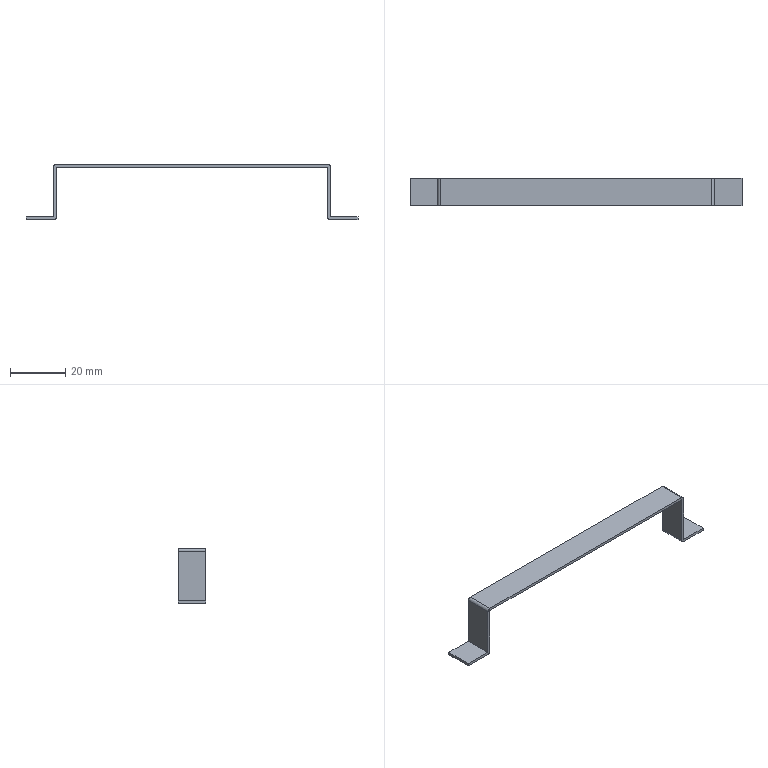Part | STEP file | RJWD-DY-0101_20001 | 1 solid | 18 faces | box 120 x 10 x 20 mm | volume 1571 mm3 | plane 14 | cylinder 4 | commonest cylinder face diameters 2.004 x3 2 x1
STEP:
#1=CARTESIAN_POINT('',(0.,0.,0.));
#2=DIRECTION('',(0.,0.,1.));
#3=DIRECTION('',(1.,0.,0.));
#4=AXIS2_PLACEMENT_3D('',#1,#2,#3);
#5=CARTESIAN_POINT('',(-930.573,5381.573,97.644));
#6=VERTEX_POINT('',#5);
#7=CARTESIAN_POINT('',(-931.573,5381.573,98.644));
#8=VERTEX_POINT('',#7);
#9=CARTESIAN_POINT('',(-931.573,5381.573,97.644));
#10=DIRECTION('',(0.,-1.,0.));
#11=DIRECTION('',(1.,0.,0.));
#12=AXIS2_PLACEMENT_3D('',#9,#10,#11);
#13=CIRCLE('',#12,1.);
#14=CARTESIAN_POINT('',(-1040.573,5381.573,97.644));
#15=DIRECTION('',(0.,-1.,0.));
#16=DIRECTION('',(0.,0.,-1.));
#17=AXIS2_PLACEMENT_3D('',#14,#15,#16);
#18=PLANE('',#17);
#19=CARTESIAN_POINT('',(0.,109.));
#20=DIRECTION('',(0.,1.));
#21=AXIS2_PLACEMENT_2D('',#19,#20);
#22=CIRCLE('',#21,1.);
#23=(GEOMETRIC_REPRESENTATION_CONTEXT(2)PARAMETRIC_REPRESENTATION_CONTEXT()REPRESENTATION_CONTEXT('',''));
#24=DEFINITIONAL_REPRESENTATION('',(#22),#23);
#25=PCURVE('',#18,#24);
#26=CARTESIAN_POINT('',(-931.573,5345.501,97.644));
#27=DIRECTION('',(0.,1.,0.));
#28=DIRECTION('',(0.,0.,1.));
#29=AXIS2_PLACEMENT_3D('',#26,#27,#28);
#30=CYLINDRICAL_SURFACE('',#29,1.);
#31=CARTESIAN_POINT('',(1.571,36.072));
#32=DIRECTION('',(-1.,0.));
#33=VECTOR('',#32,1.);
#34=LINE('',#31,#33);
#35=(GEOMETRIC_REPRESENTATION_CONTEXT(2)PARAMETRIC_REPRESENTATION_CONTEXT()REPRESENTATION_CONTEXT('',''));
#36=DEFINITIONAL_REPRESENTATION('',(#34),#35);
#37=PCURVE('',#30,#36);
#38=SURFACE_CURVE('',#13,(#25,#37),.PCURVE_S1.);
#39=EDGE_CURVE('',#6,#8,#38,.T.);
#40=ORIENTED_EDGE('',*,*,#39,.F.);
#41=CARTESIAN_POINT('',(-930.573,5381.573,79.644));
#42=VERTEX_POINT('',#41);
#43=CARTESIAN_POINT('',(-930.573,5381.573,97.644));
#44=DIRECTION('',(0.,0.,-1.));
#45=VECTOR('',#44,1.);
#46=LINE('',#43,#45);
#47=CARTESIAN_POINT('',(0.,110.));
#48=DIRECTION('',(1.,0.));
#49=VECTOR('',#48,1.);
#50=LINE('',#47,#49);
#51=(GEOMETRIC_REPRESENTATION_CONTEXT(2)PARAMETRIC_REPRESENTATION_CONTEXT()REPRESENTATION_CONTEXT('',''));
#52=DEFINITIONAL_REPRESENTATION('',(#50),#51);
#53=PCURVE('',#18,#52);
#54=CARTESIAN_POINT('',(-930.573,-10.,0.));
#55=DIRECTION('',(1.,0.,0.));
#56=DIRECTION('',(0.,0.,-1.));
#57=AXIS2_PLACEMENT_3D('',#54,#55,#56);
#58=PLANE('',#57);
#59=CARTESIAN_POINT('',(-97.644,5391.573));
#60=DIRECTION('',(1.,0.));
#61=VECTOR('',#60,1.);
#62=LINE('',#59,#61);
#63=(GEOMETRIC_REPRESENTATION_CONTEXT(2)PARAMETRIC_REPRESENTATION_CONTEXT()REPRESENTATION_CONTEXT('',''));
#64=DEFINITIONAL_REPRESENTATION('',(#62),#63);
#65=PCURVE('',#58,#64);
#66=SURFACE_CURVE('',#46,(#53,#65),.PCURVE_S1.);
#67=EDGE_CURVE('',#6,#42,#66,.T.);
#68=ORIENTED_EDGE('',*,*,#67,.T.);
#69=CARTESIAN_POINT('',(-920.573,5381.573,79.644));
#70=VERTEX_POINT('',#69);
#71=CARTESIAN_POINT('',(-920.573,5381.573,79.644));
#72=DIRECTION('',(-1.,0.,0.));
#73=VECTOR('',#72,1.);
#74=LINE('',#71,#73);
#75=CARTESIAN_POINT('',(18.,120.));
#76=DIRECTION('',(0.,-1.));
#77=VECTOR('',#76,1.);
#78=LINE('',#75,#77);
#79=(GEOMETRIC_REPRESENTATION_CONTEXT(2)PARAMETRIC_REPRESENTATION_CONTEXT()REPRESENTATION_CONTEXT('',''));
#80=DEFINITIONAL_REPRESENTATION('',(#78),#79);
#81=PCURVE('',#18,#80);
#82=CARTESIAN_POINT('',(-110.,-10.,79.644));
#83=DIRECTION('',(0.,0.,1.));
#84=DIRECTION('',(1.,0.,0.));
#85=AXIS2_PLACEMENT_3D('',#82,#83,#84);
#86=PLANE('',#85);
#87=CARTESIAN_POINT('',(-810.573,5391.573));
#88=DIRECTION('',(-1.,0.));
#89=VECTOR('',#88,1.);
#90=LINE('',#87,#89);
#91=(GEOMETRIC_REPRESENTATION_CONTEXT(2)PARAMETRIC_REPRESENTATION_CONTEXT()REPRESENTATION_CONTEXT('',''));
#92=DEFINITIONAL_REPRESENTATION('',(#90),#91);
#93=PCURVE('',#86,#92);
#94=SURFACE_CURVE('',#74,(#81,#93),.PCURVE_S1.);
#95=EDGE_CURVE('',#70,#42,#94,.T.);
#96=ORIENTED_EDGE('',*,*,#95,.F.);
#97=CARTESIAN_POINT('',(-920.573,5381.573,78.644));
#98=VERTEX_POINT('',#97);
#99=CARTESIAN_POINT('',(-920.573,5381.573,79.644));
#100=DIRECTION('',(0.,0.,-1.));
#101=VECTOR('',#100,1.);
#102=LINE('',#99,#101);
#103=CARTESIAN_POINT('',(18.,120.));
#104=DIRECTION('',(1.,0.));
#105=VECTOR('',#104,1.);
#106=LINE('',#103,#105);
#107=(GEOMETRIC_REPRESENTATION_CONTEXT(2)PARAMETRIC_REPRESENTATION_CONTEXT()REPRESENTATION_CONTEXT('',''));
#108=DEFINITIONAL_REPRESENTATION('',(#106),#107);
#109=PCURVE('',#18,#108);
#110=CARTESIAN_POINT('',(-920.573,5371.573,78.644));
#111=DIRECTION('',(1.,0.,0.));
#112=DIRECTION('',(0.,0.,-1.));
#113=AXIS2_PLACEMENT_3D('',#110,#111,#112);
#114=PLANE('',#113);
#115=CARTESIAN_POINT('',(-1.,10.));
#116=DIRECTION('',(1.,0.));
#117=VECTOR('',#116,1.);
#118=LINE('',#115,#117);
#119=(GEOMETRIC_REPRESENTATION_CONTEXT(2)PARAMETRIC_REPRESENTATION_CONTEXT()REPRESENTATION_CONTEXT('',''));
#120=DEFINITIONAL_REPRESENTATION('',(#118),#119);
#121=PCURVE('',#114,#120);
#122=SURFACE_CURVE('',#102,(#109,#121),.PCURVE_S1.);
#123=EDGE_CURVE('',#70,#98,#122,.T.);
#124=ORIENTED_EDGE('',*,*,#123,.T.);
#125=CARTESIAN_POINT('',(-930.571,5381.573,78.644));
#126=VERTEX_POINT('',#125);
#127=CARTESIAN_POINT('',(-920.573,5381.573,78.644));
#128=DIRECTION('',(-1.,0.,0.));
#129=VECTOR('',#128,1.);
#130=LINE('',#127,#129);
#131=CARTESIAN_POINT('',(19.,120.));
#132=DIRECTION('',(0.,-1.));
#133=VECTOR('',#132,1.);
#134=LINE('',#131,#133);
#135=(GEOMETRIC_REPRESENTATION_CONTEXT(2)PARAMETRIC_REPRESENTATION_CONTEXT()REPRESENTATION_CONTEXT('',''));
#136=DEFINITIONAL_REPRESENTATION('',(#134),#135);
#137=PCURVE('',#18,#136);
#138=CARTESIAN_POINT('',(-110.,-10.,78.644));
#139=DIRECTION('',(0.,0.,1.));
#140=DIRECTION('',(1.,0.,0.));
#141=AXIS2_PLACEMENT_3D('',#138,#139,#140);
#142=PLANE('',#141);
#143=CARTESIAN_POINT('',(-810.573,5391.573));
#144=DIRECTION('',(-1.,0.));
#145=VECTOR('',#144,1.);
#146=LINE('',#143,#145);
#147=(GEOMETRIC_REPRESENTATION_CONTEXT(2)PARAMETRIC_REPRESENTATION_CONTEXT()REPRESENTATION_CONTEXT('',''));
#148=DEFINITIONAL_REPRESENTATION('',(#146),#147);
#149=PCURVE('',#142,#148);
#150=SURFACE_CURVE('',#130,(#137,#149),.PCURVE_S1.);
#151=EDGE_CURVE('',#98,#126,#150,.T.);
#152=ORIENTED_EDGE('',*,*,#151,.T.);
#153=CARTESIAN_POINT('',(-931.573,5381.573,79.646));
#154=VERTEX_POINT('',#153);
#155=CARTESIAN_POINT('',(-930.571,5381.573,79.646));
#156=DIRECTION('',(0.,-1.,0.));
#157=DIRECTION('',(-1.,0.,0.));
#158=AXIS2_PLACEMENT_3D('',#155,#156,#157);
#159=CIRCLE('',#158,1.002);
#160=CARTESIAN_POINT('',(17.998,110.002));
#161=DIRECTION('',(0.,-1.));
#162=AXIS2_PLACEMENT_2D('',#160,#161);
#163=CIRCLE('',#162,1.002);
#164=(GEOMETRIC_REPRESENTATION_CONTEXT(2)PARAMETRIC_REPRESENTATION_CONTEXT()REPRESENTATION_CONTEXT('',''));
#165=DEFINITIONAL_REPRESENTATION('',(#163),#164);
#166=PCURVE('',#18,#165);
#167=CARTESIAN_POINT('',(-930.571,5411.573,79.646));
#168=DIRECTION('',(0.,-1.,0.));
#169=DIRECTION('',(1.,0.,0.));
#170=AXIS2_PLACEMENT_3D('',#167,#168,#169);
#171=CYLINDRICAL_SURFACE('',#170,1.002);
#172=CARTESIAN_POINT('',(3.142,30.));
#173=DIRECTION('',(1.,0.));
#174=VECTOR('',#173,1.);
#175=LINE('',#172,#174);
#176=(GEOMETRIC_REPRESENTATION_CONTEXT(2)PARAMETRIC_REPRESENTATION_CONTEXT()REPRESENTATION_CONTEXT('',''));
#177=DEFINITIONAL_REPRESENTATION('',(#175),#176);
#178=PCURVE('',#171,#177);
#179=SURFACE_CURVE('',#159,(#166,#178),.PCURVE_S1.);
#180=EDGE_CURVE('',#154,#126,#179,.T.);
#181=ORIENTED_EDGE('',*,*,#180,.F.);
#182=CARTESIAN_POINT('',(-931.573,5381.573,97.644));
#183=VERTEX_POINT('',#182);
#184=CARTESIAN_POINT('',(-931.573,5381.573,79.646));
#185=DIRECTION('',(0.,0.,1.));
#186=VECTOR('',#185,1.);
#187=LINE('',#184,#186);
#188=CARTESIAN_POINT('',(17.998,109.));
#189=DIRECTION('',(-1.,0.));
#190=VECTOR('',#189,1.);
#191=LINE('',#188,#190);
#192=(GEOMETRIC_REPRESENTATION_CONTEXT(2)PARAMETRIC_REPRESENTATION_CONTEXT()REPRESENTATION_CONTEXT('',''));
#193=DEFINITIONAL_REPRESENTATION('',(#191),#192);
#194=PCURVE('',#18,#193);
#195=CARTESIAN_POINT('',(-931.573,-10.,0.));
#196=DIRECTION('',(1.,0.,0.));
#197=DIRECTION('',(0.,0.,-1.));
#198=AXIS2_PLACEMENT_3D('',#195,#196,#197);
#199=PLANE('',#198);
#200=CARTESIAN_POINT('',(-79.646,5391.573));
#201=DIRECTION('',(-1.,0.));
#202=VECTOR('',#201,1.);
#203=LINE('',#200,#202);
#204=(GEOMETRIC_REPRESENTATION_CONTEXT(2)PARAMETRIC_REPRESENTATION_CONTEXT()REPRESENTATION_CONTEXT('',''));
#205=DEFINITIONAL_REPRESENTATION('',(#203),#204);
#206=PCURVE('',#199,#205);
#207=SURFACE_CURVE('',#187,(#194,#206),.PCURVE_S1.);
#208=EDGE_CURVE('',#154,#183,#207,.T.);
#209=ORIENTED_EDGE('',*,*,#208,.T.);
#210=CARTESIAN_POINT('',(-1029.573,5381.573,97.644));
#211=VERTEX_POINT('',#210);
#212=CARTESIAN_POINT('',(-931.573,5381.573,97.644));
#213=DIRECTION('',(-1.,0.,0.));
#214=VECTOR('',#213,1.);
#215=LINE('',#212,#214);
#216=CARTESIAN_POINT('',(0.,109.));
#217=DIRECTION('',(0.,-1.));
#218=VECTOR('',#217,1.);
#219=LINE('',#216,#218);
#220=(GEOMETRIC_REPRESENTATION_CONTEXT(2)PARAMETRIC_REPRESENTATION_CONTEXT()REPRESENTATION_CONTEXT('',''));
#221=DEFINITIONAL_REPRESENTATION('',(#219),#220);
#222=PCURVE('',#18,#221);
#223=CARTESIAN_POINT('',(0.,-10.,97.644));
#224=DIRECTION('',(0.,0.,1.));
#225=DIRECTION('',(1.,0.,0.));
#226=AXIS2_PLACEMENT_3D('',#223,#224,#225);
#227=PLANE('',#226);
#228=CARTESIAN_POINT('',(-931.573,5391.573));
#229=DIRECTION('',(-1.,0.));
#230=VECTOR('',#229,1.);
#231=LINE('',#228,#230);
#232=(GEOMETRIC_REPRESENTATION_CONTEXT(2)PARAMETRIC_REPRESENTATION_CONTEXT()REPRESENTATION_CONTEXT('',''));
#233=DEFINITIONAL_REPRESENTATION('',(#231),#232);
#234=PCURVE('',#227,#233);
#235=SURFACE_CURVE('',#215,(#222,#234),.PCURVE_S1.);
#236=EDGE_CURVE('',#183,#211,#235,.T.);
#237=ORIENTED_EDGE('',*,*,#236,.T.);
#238=CARTESIAN_POINT('',(-1029.573,5381.573,79.646));
#239=VERTEX_POINT('',#238);
#240=CARTESIAN_POINT('',(-1029.573,5381.573,79.646));
#241=DIRECTION('',(0.,0.,1.));
#242=VECTOR('',#241,1.);
#243=LINE('',#240,#242);
#244=CARTESIAN_POINT('',(17.998,11.));
#245=DIRECTION('',(-1.,0.));
#246=VECTOR('',#245,1.);
#247=LINE('',#244,#246);
#248=(GEOMETRIC_REPRESENTATION_CONTEXT(2)PARAMETRIC_REPRESENTATION_CONTEXT()REPRESENTATION_CONTEXT('',''));
#249=DEFINITIONAL_REPRESENTATION('',(#247),#248);
#250=PCURVE('',#18,#249);
#251=CARTESIAN_POINT('',(-1029.573,-10.,0.));
#252=DIRECTION('',(1.,0.,0.));
#253=DIRECTION('',(0.,0.,-1.));
#254=AXIS2_PLACEMENT_3D('',#251,#252,#253);
#255=PLANE('',#254);
#256=CARTESIAN_POINT('',(-79.646,5391.573));
#257=DIRECTION('',(-1.,0.));
#258=VECTOR('',#257,1.);
#259=LINE('',#256,#258);
#260=(GEOMETRIC_REPRESENTATION_CONTEXT(2)PARAMETRIC_REPRESENTATION_CONTEXT()REPRESENTATION_CONTEXT('',''));
#261=DEFINITIONAL_REPRESENTATION('',(#259),#260);
#262=PCURVE('',#255,#261);
#263=SURFACE_CURVE('',#243,(#250,#262),.PCURVE_S1.);
#264=EDGE_CURVE('',#239,#211,#263,.T.);
#265=ORIENTED_EDGE('',*,*,#264,.F.);
#266=CARTESIAN_POINT('',(-1030.575,5381.573,78.644));
#267=VERTEX_POINT('',#266);
#268=CARTESIAN_POINT('',(-1030.575,5381.573,79.646));
#269=DIRECTION('',(0.,-1.,0.));
#270=DIRECTION('',(0.,0.,-1.));
#271=AXIS2_PLACEMENT_3D('',#268,#269,#270);
#272=CIRCLE('',#271,1.002);
#273=CARTESIAN_POINT('',(17.998,9.998));
#274=DIRECTION('',(1.,0.));
#275=AXIS2_PLACEMENT_2D('',#273,#274);
#276=CIRCLE('',#275,1.002);
#277=(GEOMETRIC_REPRESENTATION_CONTEXT(2)PARAMETRIC_REPRESENTATION_CONTEXT()REPRESENTATION_CONTEXT('',''));
#278=DEFINITIONAL_REPRESENTATION('',(#276),#277);
#279=PCURVE('',#18,#278);
#280=CARTESIAN_POINT('',(-1030.575,5371.573,79.646));
#281=DIRECTION('',(0.,1.,0.));
#282=DIRECTION('',(-1.,0.,0.));
#283=AXIS2_PLACEMENT_3D('',#280,#281,#282);
#284=CYLINDRICAL_SURFACE('',#283,1.002);
#285=CARTESIAN_POINT('',(4.712,10.));
#286=DIRECTION('',(-1.,0.));
#287=VECTOR('',#286,1.);
#288=LINE('',#285,#287);
#289=(GEOMETRIC_REPRESENTATION_CONTEXT(2)PARAMETRIC_REPRESENTATION_CONTEXT()REPRESENTATION_CONTEXT('',''));
#290=DEFINITIONAL_REPRESENTATION('',(#288),#289);
#291=PCURVE('',#284,#290);
#292=SURFACE_CURVE('',#272,(#279,#291),.PCURVE_S1.);
#293=EDGE_CURVE('',#267,#239,#292,.T.);
#294=ORIENTED_EDGE('',*,*,#293,.F.);
#295=CARTESIAN_POINT('',(-1040.573,5381.573,78.644));
#296=VERTEX_POINT('',#295);
#297=CARTESIAN_POINT('',(-1040.573,5381.573,78.644));
#298=DIRECTION('',(1.,0.,0.));
#299=VECTOR('',#298,1.);
#300=LINE('',#297,#299);
#301=CARTESIAN_POINT('',(19.,0.));
#302=DIRECTION('',(0.,1.));
#303=VECTOR('',#302,1.);
#304=LINE('',#301,#303);
#305=(GEOMETRIC_REPRESENTATION_CONTEXT(2)PARAMETRIC_REPRESENTATION_CONTEXT()REPRESENTATION_CONTEXT('',''));
#306=DEFINITIONAL_REPRESENTATION('',(#304),#305);
#307=PCURVE('',#18,#306);
#308=CARTESIAN_POINT('',(10.,-10.,78.644));
#309=DIRECTION('',(0.,0.,-1.));
#310=DIRECTION('',(-1.,0.,0.));
#311=AXIS2_PLACEMENT_3D('',#308,#309,#310);
#312=PLANE('',#311);
#313=CARTESIAN_POINT('',(1050.573,5391.573));
#314=DIRECTION('',(-1.,0.));
#315=VECTOR('',#314,1.);
#316=LINE('',#313,#315);
#317=(GEOMETRIC_REPRESENTATION_CONTEXT(2)PARAMETRIC_REPRESENTATION_CONTEXT()REPRESENTATION_CONTEXT('',''));
#318=DEFINITIONAL_REPRESENTATION('',(#316),#317);
#319=PCURVE('',#312,#318);
#320=SURFACE_CURVE('',#300,(#307,#319),.PCURVE_S1.);
#321=EDGE_CURVE('',#296,#267,#320,.T.);
#322=ORIENTED_EDGE('',*,*,#321,.F.);
#323=CARTESIAN_POINT('',(-1040.573,5381.573,79.644));
#324=VERTEX_POINT('',#323);
#325=CARTESIAN_POINT('',(-1040.573,5381.573,79.644));
#326=DIRECTION('',(0.,0.,-1.));
#327=VECTOR('',#326,1.);
#328=LINE('',#325,#327);
#329=CARTESIAN_POINT('',(18.,0.));
#330=DIRECTION('',(1.,0.));
#331=VECTOR('',#330,1.);
#332=LINE('',#329,#331);
#333=(GEOMETRIC_REPRESENTATION_CONTEXT(2)PARAMETRIC_REPRESENTATION_CONTEXT()REPRESENTATION_CONTEXT('',''));
#334=DEFINITIONAL_REPRESENTATION('',(#332),#333);
#335=PCURVE('',#18,#334);
#336=CARTESIAN_POINT('',(-1040.573,5371.573,78.644));
#337=DIRECTION('',(1.,0.,0.));
#338=DIRECTION('',(0.,0.,-1.));
#339=AXIS2_PLACEMENT_3D('',#336,#337,#338);
#340=PLANE('',#339);
#341=CARTESIAN_POINT('',(-1.,10.));
#342=DIRECTION('',(1.,0.));
#343=VECTOR('',#342,1.);
#344=LINE('',#341,#343);
#345=(GEOMETRIC_REPRESENTATION_CONTEXT(2)PARAMETRIC_REPRESENTATION_CONTEXT()REPRESENTATION_CONTEXT('',''));
#346=DEFINITIONAL_REPRESENTATION('',(#344),#345);
#347=PCURVE('',#340,#346);
#348=SURFACE_CURVE('',#328,(#335,#347),.PCURVE_S1.);
#349=EDGE_CURVE('',#324,#296,#348,.T.);
#350=ORIENTED_EDGE('',*,*,#349,.F.);
#351=CARTESIAN_POINT('',(-1030.573,5381.573,79.644));
#352=VERTEX_POINT('',#351);
#353=CARTESIAN_POINT('',(-1040.573,5381.573,79.644));
#354=DIRECTION('',(1.,0.,0.));
#355=VECTOR('',#354,1.);
#356=LINE('',#353,#355);
#357=CARTESIAN_POINT('',(18.,0.));
#358=DIRECTION('',(0.,1.));
#359=VECTOR('',#358,1.);
#360=LINE('',#357,#359);
#361=(GEOMETRIC_REPRESENTATION_CONTEXT(2)PARAMETRIC_REPRESENTATION_CONTEXT()REPRESENTATION_CONTEXT('',''));
#362=DEFINITIONAL_REPRESENTATION('',(#360),#361);
#363=PCURVE('',#18,#362);
#364=CARTESIAN_POINT('',(10.,-10.,79.644));
#365=DIRECTION('',(0.,0.,-1.));
#366=DIRECTION('',(-1.,0.,0.));
#367=AXIS2_PLACEMENT_3D('',#364,#365,#366);
#368=PLANE('',#367);
#369=CARTESIAN_POINT('',(1050.573,5391.573));
#370=DIRECTION('',(-1.,0.));
#371=VECTOR('',#370,1.);
#372=LINE('',#369,#371);
#373=(GEOMETRIC_REPRESENTATION_CONTEXT(2)PARAMETRIC_REPRESENTATION_CONTEXT()REPRESENTATION_CONTEXT('',''));
#374=DEFINITIONAL_REPRESENTATION('',(#372),#373);
#375=PCURVE('',#368,#374);
#376=SURFACE_CURVE('',#356,(#363,#375),.PCURVE_S1.);
#377=EDGE_CURVE('',#324,#352,#376,.T.);
#378=ORIENTED_EDGE('',*,*,#377,.T.);
#379=CARTESIAN_POINT('',(-1030.573,5381.573,97.642));
#380=VERTEX_POINT('',#379);
#381=CARTESIAN_POINT('',(-1030.573,5381.573,79.644));
#382=DIRECTION('',(0.,0.,1.));
#383=VECTOR('',#382,1.);
#384=LINE('',#381,#383);
#385=CARTESIAN_POINT('',(18.,10.));
#386=DIRECTION('',(-1.,0.));
#387=VECTOR('',#386,1.);
#388=LINE('',#385,#387);
#389=(GEOMETRIC_REPRESENTATION_CONTEXT(2)PARAMETRIC_REPRESENTATION_CONTEXT()REPRESENTATION_CONTEXT('',''));
#390=DEFINITIONAL_REPRESENTATION('',(#388),#389);
#391=PCURVE('',#18,#390);
#392=CARTESIAN_POINT('',(-1030.573,-10.,0.));
#393=DIRECTION('',(1.,0.,0.));
#394=DIRECTION('',(0.,0.,-1.));
#395=AXIS2_PLACEMENT_3D('',#392,#393,#394);
#396=PLANE('',#395);
#397=CARTESIAN_POINT('',(-79.644,5391.573));
#398=DIRECTION('',(-1.,0.));
#399=VECTOR('',#398,1.);
#400=LINE('',#397,#399);
#401=(GEOMETRIC_REPRESENTATION_CONTEXT(2)PARAMETRIC_REPRESENTATION_CONTEXT()REPRESENTATION_CONTEXT('',''));
#402=DEFINITIONAL_REPRESENTATION('',(#400),#401);
#403=PCURVE('',#396,#402);
#404=SURFACE_CURVE('',#384,(#391,#403),.PCURVE_S1.);
#405=EDGE_CURVE('',#352,#380,#404,.T.);
#406=ORIENTED_EDGE('',*,*,#405,.T.);
#407=CARTESIAN_POINT('',(-1029.571,5381.573,98.644));
#408=VERTEX_POINT('',#407);
#409=CARTESIAN_POINT('',(-1029.571,5381.573,97.642));
#410=DIRECTION('',(0.,-1.,0.));
#411=DIRECTION('',(0.,0.,1.));
#412=AXIS2_PLACEMENT_3D('',#409,#410,#411);
#413=CIRCLE('',#412,1.002);
#414=CARTESIAN_POINT('',(0.002,11.002));
#415=DIRECTION('',(-1.,0.));
#416=AXIS2_PLACEMENT_2D('',#414,#415);
#417=CIRCLE('',#416,1.002);
#418=(GEOMETRIC_REPRESENTATION_CONTEXT(2)PARAMETRIC_REPRESENTATION_CONTEXT()REPRESENTATION_CONTEXT('',''));
#419=DEFINITIONAL_REPRESENTATION('',(#417),#418);
#420=PCURVE('',#18,#419);
#421=CARTESIAN_POINT('',(-1029.571,5411.573,97.642));
#422=DIRECTION('',(0.,-1.,0.));
#423=DIRECTION('',(0.,0.,-1.));
#424=AXIS2_PLACEMENT_3D('',#421,#422,#423);
#425=CYLINDRICAL_SURFACE('',#424,1.002);
#426=CARTESIAN_POINT('',(3.142,30.));
#427=DIRECTION('',(1.,0.));
#428=VECTOR('',#427,1.);
#429=LINE('',#426,#428);
#430=(GEOMETRIC_REPRESENTATION_CONTEXT(2)PARAMETRIC_REPRESENTATION_CONTEXT()REPRESENTATION_CONTEXT('',''));
#431=DEFINITIONAL_REPRESENTATION('',(#429),#430);
#432=PCURVE('',#425,#431);
#433=SURFACE_CURVE('',#413,(#420,#432),.PCURVE_S1.);
#434=EDGE_CURVE('',#408,#380,#433,.T.);
#435=ORIENTED_EDGE('',*,*,#434,.F.);
#436=CARTESIAN_POINT('',(-1029.571,5381.573,98.644));
#437=DIRECTION('',(1.,0.,0.));
#438=VECTOR('',#437,1.);
#439=LINE('',#436,#438);
#440=CARTESIAN_POINT('',(-1.,11.002));
#441=DIRECTION('',(0.,1.));
#442=VECTOR('',#441,1.);
#443=LINE('',#440,#442);
#444=(GEOMETRIC_REPRESENTATION_CONTEXT(2)PARAMETRIC_REPRESENTATION_CONTEXT()REPRESENTATION_CONTEXT('',''));
#445=DEFINITIONAL_REPRESENTATION('',(#443),#444);
#446=PCURVE('',#18,#445);
#447=CARTESIAN_POINT('',(0.,-10.,98.644));
#448=DIRECTION('',(0.,0.,1.));
#449=DIRECTION('',(1.,0.,0.));
#450=AXIS2_PLACEMENT_3D('',#447,#448,#449);
#451=PLANE('',#450);
#452=CARTESIAN_POINT('',(-1029.571,5391.573));
#453=DIRECTION('',(1.,0.));
#454=VECTOR('',#453,1.);
#455=LINE('',#452,#454);
#456=(GEOMETRIC_REPRESENTATION_CONTEXT(2)PARAMETRIC_REPRESENTATION_CONTEXT()REPRESENTATION_CONTEXT('',''));
#457=DEFINITIONAL_REPRESENTATION('',(#455),#456);
#458=PCURVE('',#451,#457);
#459=SURFACE_CURVE('',#439,(#446,#458),.PCURVE_S1.);
#460=EDGE_CURVE('',#408,#8,#459,.T.);
#461=ORIENTED_EDGE('',*,*,#460,.T.);
#462=EDGE_LOOP('',(#40,#68,#96,#124,#152,#181,#209,#237,#265,#294,#322,#350,#378,#406,#435,#461));
#463=FACE_BOUND('',#462,.F.);
#464=ADVANCED_FACE('',(#463),#18,.T.);
#465=CARTESIAN_POINT('',(-931.573,5391.573,98.644));
#466=VERTEX_POINT('',#465);
#467=CARTESIAN_POINT('',(-931.573,5381.573,98.644));
#468=DIRECTION('',(0.,1.,0.));
#469=VECTOR('',#468,1.);
#470=LINE('',#467,#469);
#471=CARTESIAN_POINT('',(0.,36.072));
#472=DIRECTION('',(0.,1.));
#473=VECTOR('',#472,1.);
#474=LINE('',#471,#473);
#475=(GEOMETRIC_REPRESENTATION_CONTEXT(2)PARAMETRIC_REPRESENTATION_CONTEXT()REPRESENTATION_CONTEXT('',''));
#476=DEFINITIONAL_REPRESENTATION('',(#474),#475);
#477=PCURVE('',#30,#476);
#478=CARTESIAN_POINT('',(-931.573,5391.573));
#479=DIRECTION('',(0.,1.));
#480=VECTOR('',#479,1.);
#481=LINE('',#478,#480);
#482=(GEOMETRIC_REPRESENTATION_CONTEXT(2)PARAMETRIC_REPRESENTATION_CONTEXT()REPRESENTATION_CONTEXT('',''));
#483=DEFINITIONAL_REPRESENTATION('',(#481),#482);
#484=PCURVE('',#451,#483);
#485=SURFACE_CURVE('',#470,(#477,#484),.PCURVE_S1.);
#486=EDGE_CURVE('',#8,#466,#485,.T.);
#487=ORIENTED_EDGE('',*,*,#486,.F.);
#488=ORIENTED_EDGE('',*,*,#39,.F.);
#489=CARTESIAN_POINT('',(-930.573,5391.573,97.644));
#490=VERTEX_POINT('',#489);
#491=CARTESIAN_POINT('',(-930.573,5381.573,97.644));
#492=DIRECTION('',(0.,1.,0.));
#493=VECTOR('',#492,1.);
#494=LINE('',#491,#493);
#495=CARTESIAN_POINT('',(1.571,36.072));
#496=DIRECTION('',(0.,1.));
#497=VECTOR('',#496,1.);
#498=LINE('',#495,#497);
#499=(GEOMETRIC_REPRESENTATION_CONTEXT(2)PARAMETRIC_REPRESENTATION_CONTEXT()REPRESENTATION_CONTEXT('',''));
#500=DEFINITIONAL_REPRESENTATION('',(#498),#499);
#501=PCURVE('',#30,#500);
#502=CARTESIAN_POINT('',(-97.644,5391.573));
#503=DIRECTION('',(0.,1.));
#504=VECTOR('',#503,1.);
#505=LINE('',#502,#504);
#506=(GEOMETRIC_REPRESENTATION_CONTEXT(2)PARAMETRIC_REPRESENTATION_CONTEXT()REPRESENTATION_CONTEXT('',''));
#507=DEFINITIONAL_REPRESENTATION('',(#505),#506);
#508=PCURVE('',#58,#507);
#509=SURFACE_CURVE('',#494,(#501,#508),.PCURVE_S1.);
#510=EDGE_CURVE('',#6,#490,#509,.T.);
#511=ORIENTED_EDGE('',*,*,#510,.T.);
#512=CARTESIAN_POINT('',(-931.573,5391.573,97.644));
#513=DIRECTION('',(0.,1.,0.));
#514=DIRECTION('',(0.,0.,1.));
#515=AXIS2_PLACEMENT_3D('',#512,#513,#514);
#516=CIRCLE('',#515,1.);
#517=CARTESIAN_POINT('',(0.,46.072));
#518=DIRECTION('',(1.,0.));
#519=VECTOR('',#518,1.);
#520=LINE('',#517,#519);
#521=(GEOMETRIC_REPRESENTATION_CONTEXT(2)PARAMETRIC_REPRESENTATION_CONTEXT()REPRESENTATION_CONTEXT('',''));
#522=DEFINITIONAL_REPRESENTATION('',(#520),#521);
#523=PCURVE('',#30,#522);
#524=CARTESIAN_POINT('',(-820.573,5391.573,97.644));
#525=DIRECTION('',(0.,1.,0.));
#526=DIRECTION('',(0.,0.,1.));
#527=AXIS2_PLACEMENT_3D('',#524,#525,#526);
#528=PLANE('',#527);
#529=CARTESIAN_POINT('',(0.,-111.));
#530=DIRECTION('',(1.,0.));
#531=AXIS2_PLACEMENT_2D('',#529,#530);
#532=CIRCLE('',#531,1.);
#533=(GEOMETRIC_REPRESENTATION_CONTEXT(2)PARAMETRIC_REPRESENTATION_CONTEXT()REPRESENTATION_CONTEXT('',''));
#534=DEFINITIONAL_REPRESENTATION('',(#532),#533);
#535=PCURVE('',#528,#534);
#536=SURFACE_CURVE('',#516,(#523,#535),.PCURVE_S1.);
#537=EDGE_CURVE('',#466,#490,#536,.T.);
#538=ORIENTED_EDGE('',*,*,#537,.F.);
#539=EDGE_LOOP('',(#487,#488,#511,#538));
#540=FACE_BOUND('',#539,.T.);
#541=ADVANCED_FACE('',(#540),#30,.T.);
#542=ORIENTED_EDGE('',*,*,#537,.F.);
#543=CARTESIAN_POINT('',(-1029.571,5391.573,98.644));
#544=VERTEX_POINT('',#543);
#545=CARTESIAN_POINT('',(-931.573,5391.573,98.644));
#546=DIRECTION('',(-1.,0.,0.));
#547=VECTOR('',#546,1.);
#548=LINE('',#545,#547);
#549=CARTESIAN_POINT('',(1.,-111.));
#550=DIRECTION('',(0.,-1.));
#551=VECTOR('',#550,1.);
#552=LINE('',#549,#551);
#553=(GEOMETRIC_REPRESENTATION_CONTEXT(2)PARAMETRIC_REPRESENTATION_CONTEXT()REPRESENTATION_CONTEXT('',''));
#554=DEFINITIONAL_REPRESENTATION('',(#552),#553);
#555=PCURVE('',#528,#554);
#556=CARTESIAN_POINT('',(-931.573,5401.573));
#557=DIRECTION('',(-1.,0.));
#558=VECTOR('',#557,1.);
#559=LINE('',#556,#558);
#560=(GEOMETRIC_REPRESENTATION_CONTEXT(2)PARAMETRIC_REPRESENTATION_CONTEXT()REPRESENTATION_CONTEXT('',''));
#561=DEFINITIONAL_REPRESENTATION('',(#559),#560);
#562=PCURVE('',#451,#561);
#563=SURFACE_CURVE('',#548,(#555,#562),.PCURVE_S1.);
#564=EDGE_CURVE('',#466,#544,#563,.T.);
#565=ORIENTED_EDGE('',*,*,#564,.T.);
#566=CARTESIAN_POINT('',(-1030.573,5391.573,97.642));
#567=VERTEX_POINT('',#566);
#568=CARTESIAN_POINT('',(-1029.571,5391.573,97.642));
#569=DIRECTION('',(0.,1.,0.));
#570=DIRECTION('',(-1.,0.,0.));
#571=AXIS2_PLACEMENT_3D('',#568,#569,#570);
#572=CIRCLE('',#571,1.002);
#573=CARTESIAN_POINT('',(-0.002,-208.998));
#574=DIRECTION('',(0.,-1.));
#575=AXIS2_PLACEMENT_2D('',#573,#574);
#576=CIRCLE('',#575,1.002);
#577=(GEOMETRIC_REPRESENTATION_CONTEXT(2)PARAMETRIC_REPRESENTATION_CONTEXT()REPRESENTATION_CONTEXT('',''));
#578=DEFINITIONAL_REPRESENTATION('',(#576),#577);
#579=PCURVE('',#528,#578);
#580=CARTESIAN_POINT('',(4.712,20.));
#581=DIRECTION('',(-1.,0.));
#582=VECTOR('',#581,1.);
#583=LINE('',#580,#582);
#584=(GEOMETRIC_REPRESENTATION_CONTEXT(2)PARAMETRIC_REPRESENTATION_CONTEXT()REPRESENTATION_CONTEXT('',''));
#585=DEFINITIONAL_REPRESENTATION('',(#583),#584);
#586=PCURVE('',#425,#585);
#587=SURFACE_CURVE('',#572,(#579,#586),.PCURVE_S1.);
#588=EDGE_CURVE('',#567,#544,#587,.T.);
#589=ORIENTED_EDGE('',*,*,#588,.F.);
#590=CARTESIAN_POINT('',(-1030.573,5391.573,79.644));
#591=VERTEX_POINT('',#590);
#592=CARTESIAN_POINT('',(-1030.573,5391.573,97.642));
#593=DIRECTION('',(-0.00003704,0.,-1.));
#594=VECTOR('',#593,1.);
#595=LINE('',#592,#594);
#596=CARTESIAN_POINT('',(-0.002,-210.));
#597=DIRECTION('',(-1.,-0.00003704));
#598=VECTOR('',#597,1.);
#599=LINE('',#596,#598);
#600=(GEOMETRIC_REPRESENTATION_CONTEXT(2)PARAMETRIC_REPRESENTATION_CONTEXT()REPRESENTATION_CONTEXT('',''));
#601=DEFINITIONAL_REPRESENTATION('',(#599),#600);
#602=PCURVE('',#528,#601);
#603=CARTESIAN_POINT('',(-97.642,5401.573));
#604=DIRECTION('',(1.,0.));
#605=VECTOR('',#604,1.);
#606=LINE('',#603,#605);
#607=(GEOMETRIC_REPRESENTATION_CONTEXT(2)PARAMETRIC_REPRESENTATION_CONTEXT()REPRESENTATION_CONTEXT('',''));
#608=DEFINITIONAL_REPRESENTATION('',(#606),#607);
#609=PCURVE('',#396,#608);
#610=SURFACE_CURVE('',#595,(#602,#609),.PCURVE_S1.);
#611=EDGE_CURVE('',#567,#591,#610,.T.);
#612=ORIENTED_EDGE('',*,*,#611,.T.);
#613=CARTESIAN_POINT('',(-1040.573,5391.573,79.644));
#614=VERTEX_POINT('',#613);
#615=CARTESIAN_POINT('',(-1030.573,5391.573,79.644));
#616=DIRECTION('',(-1.,0.,-0.00006667));
#617=VECTOR('',#616,1.);
#618=LINE('',#615,#617);
#619=CARTESIAN_POINT('',(-17.999,-210.001));
#620=DIRECTION('',(-0.00006667,-1.));
#621=VECTOR('',#620,1.);
#622=LINE('',#619,#621);
#623=(GEOMETRIC_REPRESENTATION_CONTEXT(2)PARAMETRIC_REPRESENTATION_CONTEXT()REPRESENTATION_CONTEXT('',''));
#624=DEFINITIONAL_REPRESENTATION('',(#622),#623);
#625=PCURVE('',#528,#624);
#626=CARTESIAN_POINT('',(1040.573,5401.573));
#627=DIRECTION('',(1.,0.));
#628=VECTOR('',#627,1.);
#629=LINE('',#626,#628);
#630=(GEOMETRIC_REPRESENTATION_CONTEXT(2)PARAMETRIC_REPRESENTATION_CONTEXT()REPRESENTATION_CONTEXT('',''));
#631=DEFINITIONAL_REPRESENTATION('',(#629),#630);
#632=PCURVE('',#368,#631);
#633=SURFACE_CURVE('',#618,(#625,#632),.PCURVE_S1.);
#634=EDGE_CURVE('',#591,#614,#633,.T.);
#635=ORIENTED_EDGE('',*,*,#634,.T.);
#636=CARTESIAN_POINT('',(-1040.573,5391.573,78.644));
#637=VERTEX_POINT('',#636);
#638=CARTESIAN_POINT('',(-1040.573,5391.573,79.644));
#639=DIRECTION('',(0.,0.,-1.));
#640=VECTOR('',#639,1.);
#641=LINE('',#638,#640);
#642=CARTESIAN_POINT('',(-18.,-220.));
#643=DIRECTION('',(-1.,0.));
#644=VECTOR('',#643,1.);
#645=LINE('',#642,#644);
#646=(GEOMETRIC_REPRESENTATION_CONTEXT(2)PARAMETRIC_REPRESENTATION_CONTEXT()REPRESENTATION_CONTEXT('',''));
#647=DEFINITIONAL_REPRESENTATION('',(#645),#646);
#648=PCURVE('',#528,#647);
#649=CARTESIAN_POINT('',(-1.,20.));
#650=DIRECTION('',(1.,0.));
#651=VECTOR('',#650,1.);
#652=LINE('',#649,#651);
#653=(GEOMETRIC_REPRESENTATION_CONTEXT(2)PARAMETRIC_REPRESENTATION_CONTEXT()REPRESENTATION_CONTEXT('',''));
#654=DEFINITIONAL_REPRESENTATION('',(#652),#653);
#655=PCURVE('',#340,#654);
#656=SURFACE_CURVE('',#641,(#648,#655),.PCURVE_S1.);
#657=EDGE_CURVE('',#614,#637,#656,.T.);
#658=ORIENTED_EDGE('',*,*,#657,.T.);
#659=CARTESIAN_POINT('',(-1030.575,5391.573,78.644));
#660=VERTEX_POINT('',#659);
#661=CARTESIAN_POINT('',(-1030.575,5391.573,78.644));
#662=DIRECTION('',(-1.,0.,0.));
#663=VECTOR('',#662,1.);
#664=LINE('',#661,#663);
#665=CARTESIAN_POINT('',(-19.,-210.002));
#666=DIRECTION('',(0.,-1.));
#667=VECTOR('',#666,1.);
#668=LINE('',#665,#667);
#669=(GEOMETRIC_REPRESENTATION_CONTEXT(2)PARAMETRIC_REPRESENTATION_CONTEXT()REPRESENTATION_CONTEXT('',''));
#670=DEFINITIONAL_REPRESENTATION('',(#668),#669);
#671=PCURVE('',#528,#670);
#672=CARTESIAN_POINT('',(1040.575,5401.573));
#673=DIRECTION('',(1.,0.));
#674=VECTOR('',#673,1.);
#675=LINE('',#672,#674);
#676=(GEOMETRIC_REPRESENTATION_CONTEXT(2)PARAMETRIC_REPRESENTATION_CONTEXT()REPRESENTATION_CONTEXT('',''));
#677=DEFINITIONAL_REPRESENTATION('',(#675),#676);
#678=PCURVE('',#312,#677);
#679=SURFACE_CURVE('',#664,(#671,#678),.PCURVE_S1.);
#680=EDGE_CURVE('',#660,#637,#679,.T.);
#681=ORIENTED_EDGE('',*,*,#680,.F.);
#682=CARTESIAN_POINT('',(-1029.573,5391.573,79.646));
#683=VERTEX_POINT('',#682);
#684=CARTESIAN_POINT('',(-1030.575,5391.573,79.646));
#685=DIRECTION('',(0.,1.,0.));
#686=DIRECTION('',(1.,0.,0.));
#687=AXIS2_PLACEMENT_3D('',#684,#685,#686);
#688=CIRCLE('',#687,1.002);
#689=CARTESIAN_POINT('',(-17.998,-210.002));
#690=DIRECTION('',(0.,1.));
#691=AXIS2_PLACEMENT_2D('',#689,#690);
#692=CIRCLE('',#691,1.002);
#693=(GEOMETRIC_REPRESENTATION_CONTEXT(2)PARAMETRIC_REPRESENTATION_CONTEXT()REPRESENTATION_CONTEXT('',''));
#694=DEFINITIONAL_REPRESENTATION('',(#692),#693);
#695=PCURVE('',#528,#694);
#696=CARTESIAN_POINT('',(3.142,20.));
#697=DIRECTION('',(1.,0.));
#698=VECTOR('',#697,1.);
#699=LINE('',#696,#698);
#700=(GEOMETRIC_REPRESENTATION_CONTEXT(2)PARAMETRIC_REPRESENTATION_CONTEXT()REPRESENTATION_CONTEXT('',''));
#701=DEFINITIONAL_REPRESENTATION('',(#699),#700);
#702=PCURVE('',#284,#701);
#703=SURFACE_CURVE('',#688,(#695,#702),.PCURVE_S1.);
#704=EDGE_CURVE('',#683,#660,#703,.T.);
#705=ORIENTED_EDGE('',*,*,#704,.F.);
#706=CARTESIAN_POINT('',(-1029.572,5391.573,97.643));
#707=VERTEX_POINT('',#706);
#708=CARTESIAN_POINT('',(-1029.572,5391.573,97.643));
#709=DIRECTION('',(-0.00003704,0.,-1.));
#710=VECTOR('',#709,1.);
#711=LINE('',#708,#710);
#712=CARTESIAN_POINT('',(-0.0006667,-208.999));
#713=DIRECTION('',(-1.,-0.00003704));
#714=VECTOR('',#713,1.);
#715=LINE('',#712,#714);
#716=(GEOMETRIC_REPRESENTATION_CONTEXT(2)PARAMETRIC_REPRESENTATION_CONTEXT()REPRESENTATION_CONTEXT('',''));
#717=DEFINITIONAL_REPRESENTATION('',(#715),#716);
#718=PCURVE('',#528,#717);
#719=CARTESIAN_POINT('',(-97.643,5401.573));
#720=DIRECTION('',(1.,0.));
#721=VECTOR('',#720,1.);
#722=LINE('',#719,#721);
#723=(GEOMETRIC_REPRESENTATION_CONTEXT(2)PARAMETRIC_REPRESENTATION_CONTEXT()REPRESENTATION_CONTEXT('',''));
#724=DEFINITIONAL_REPRESENTATION('',(#722),#723);
#725=PCURVE('',#255,#724);
#726=SURFACE_CURVE('',#711,(#718,#725),.PCURVE_S1.);
#727=EDGE_CURVE('',#707,#683,#726,.T.);
#728=ORIENTED_EDGE('',*,*,#727,.F.);
#729=CARTESIAN_POINT('',(-931.573,5391.573,97.644));
#730=VERTEX_POINT('',#729);
#731=CARTESIAN_POINT('',(-1029.572,5391.573,97.643));
#732=DIRECTION('',(1.,0.,0.000006803));
#733=VECTOR('',#732,1.);
#734=LINE('',#731,#733);
#735=CARTESIAN_POINT('',(-0.0006667,-208.999));
#736=DIRECTION('',(0.000006803,1.));
#737=VECTOR('',#736,1.);
#738=LINE('',#735,#737);
#739=(GEOMETRIC_REPRESENTATION_CONTEXT(2)PARAMETRIC_REPRESENTATION_CONTEXT()REPRESENTATION_CONTEXT('',''));
#740=DEFINITIONAL_REPRESENTATION('',(#738),#739);
#741=PCURVE('',#528,#740);
#742=CARTESIAN_POINT('',(-1029.572,5401.573));
#743=DIRECTION('',(1.,0.));
#744=VECTOR('',#743,1.);
#745=LINE('',#742,#744);
#746=(GEOMETRIC_REPRESENTATION_CONTEXT(2)PARAMETRIC_REPRESENTATION_CONTEXT()REPRESENTATION_CONTEXT('',''));
#747=DEFINITIONAL_REPRESENTATION('',(#745),#746);
#748=PCURVE('',#227,#747);
#749=SURFACE_CURVE('',#734,(#741,#748),.PCURVE_S1.);
#750=EDGE_CURVE('',#707,#730,#749,.T.);
#751=ORIENTED_EDGE('',*,*,#750,.T.);
#752=CARTESIAN_POINT('',(-931.573,5391.573,79.646));
#753=VERTEX_POINT('',#752);
#754=CARTESIAN_POINT('',(-931.573,5391.573,97.644));
#755=DIRECTION('',(0.,0.,-1.));
#756=VECTOR('',#755,1.);
#757=LINE('',#754,#756);
#758=CARTESIAN_POINT('',(0.,-111.));
#759=DIRECTION('',(-1.,0.));
#760=VECTOR('',#759,1.);
#761=LINE('',#758,#760);
#762=(GEOMETRIC_REPRESENTATION_CONTEXT(2)PARAMETRIC_REPRESENTATION_CONTEXT()REPRESENTATION_CONTEXT('',''));
#763=DEFINITIONAL_REPRESENTATION('',(#761),#762);
#764=PCURVE('',#528,#763);
#765=CARTESIAN_POINT('',(-97.644,5401.573));
#766=DIRECTION('',(1.,0.));
#767=VECTOR('',#766,1.);
#768=LINE('',#765,#767);
#769=(GEOMETRIC_REPRESENTATION_CONTEXT(2)PARAMETRIC_REPRESENTATION_CONTEXT()REPRESENTATION_CONTEXT('',''));
#770=DEFINITIONAL_REPRESENTATION('',(#768),#769);
#771=PCURVE('',#199,#770);
#772=SURFACE_CURVE('',#757,(#764,#771),.PCURVE_S1.);
#773=EDGE_CURVE('',#730,#753,#772,.T.);
#774=ORIENTED_EDGE('',*,*,#773,.T.);
#775=CARTESIAN_POINT('',(-930.571,5391.573,78.644));
#776=VERTEX_POINT('',#775);
#777=CARTESIAN_POINT('',(-930.571,5391.573,79.646));
#778=DIRECTION('',(0.,1.,0.));
#779=DIRECTION('',(0.,0.,-1.));
#780=AXIS2_PLACEMENT_3D('',#777,#778,#779);
#781=CIRCLE('',#780,1.002);
#782=CARTESIAN_POINT('',(-17.998,-109.998));
#783=DIRECTION('',(-1.,0.));
#784=AXIS2_PLACEMENT_2D('',#782,#783);
#785=CIRCLE('',#784,1.002);
#786=(GEOMETRIC_REPRESENTATION_CONTEXT(2)PARAMETRIC_REPRESENTATION_CONTEXT()REPRESENTATION_CONTEXT('',''));
#787=DEFINITIONAL_REPRESENTATION('',(#785),#786);
#788=PCURVE('',#528,#787);
#789=CARTESIAN_POINT('',(4.712,20.));
#790=DIRECTION('',(-1.,0.));
#791=VECTOR('',#790,1.);
#792=LINE('',#789,#791);
#793=(GEOMETRIC_REPRESENTATION_CONTEXT(2)PARAMETRIC_REPRESENTATION_CONTEXT()REPRESENTATION_CONTEXT('',''));
#794=DEFINITIONAL_REPRESENTATION('',(#792),#793);
#795=PCURVE('',#171,#794);
#796=SURFACE_CURVE('',#781,(#788,#795),.PCURVE_S1.);
#797=EDGE_CURVE('',#776,#753,#796,.T.);
#798=ORIENTED_EDGE('',*,*,#797,.F.);
#799=CARTESIAN_POINT('',(-920.573,5391.573,78.644));
#800=VERTEX_POINT('',#799);
#801=CARTESIAN_POINT('',(-930.571,5391.573,78.644));
#802=DIRECTION('',(1.,0.,0.));
#803=VECTOR('',#802,1.);
#804=LINE('',#801,#803);
#805=CARTESIAN_POINT('',(-19.,-109.998));
#806=DIRECTION('',(0.,1.));
#807=VECTOR('',#806,1.);
#808=LINE('',#805,#807);
#809=(GEOMETRIC_REPRESENTATION_CONTEXT(2)PARAMETRIC_REPRESENTATION_CONTEXT()REPRESENTATION_CONTEXT('',''));
#810=DEFINITIONAL_REPRESENTATION('',(#808),#809);
#811=PCURVE('',#528,#810);
#812=CARTESIAN_POINT('',(-820.571,5401.573));
#813=DIRECTION('',(1.,0.));
#814=VECTOR('',#813,1.);
#815=LINE('',#812,#814);
#816=(GEOMETRIC_REPRESENTATION_CONTEXT(2)PARAMETRIC_REPRESENTATION_CONTEXT()REPRESENTATION_CONTEXT('',''));
#817=DEFINITIONAL_REPRESENTATION('',(#815),#816);
#818=PCURVE('',#142,#817);
#819=SURFACE_CURVE('',#804,(#811,#818),.PCURVE_S1.);
#820=EDGE_CURVE('',#776,#800,#819,.T.);
#821=ORIENTED_EDGE('',*,*,#820,.T.);
#822=CARTESIAN_POINT('',(-920.573,5391.573,79.644));
#823=VERTEX_POINT('',#822);
#824=CARTESIAN_POINT('',(-920.573,5391.573,79.644));
#825=DIRECTION('',(0.,0.,-1.));
#826=VECTOR('',#825,1.);
#827=LINE('',#824,#826);
#828=CARTESIAN_POINT('',(-18.,-100.));
#829=DIRECTION('',(-1.,0.));
#830=VECTOR('',#829,1.);
#831=LINE('',#828,#830);
#832=(GEOMETRIC_REPRESENTATION_CONTEXT(2)PARAMETRIC_REPRESENTATION_CONTEXT()REPRESENTATION_CONTEXT('',''));
#833=DEFINITIONAL_REPRESENTATION('',(#831),#832);
#834=PCURVE('',#528,#833);
#835=CARTESIAN_POINT('',(-1.,20.));
#836=DIRECTION('',(1.,0.));
#837=VECTOR('',#836,1.);
#838=LINE('',#835,#837);
#839=(GEOMETRIC_REPRESENTATION_CONTEXT(2)PARAMETRIC_REPRESENTATION_CONTEXT()REPRESENTATION_CONTEXT('',''));
#840=DEFINITIONAL_REPRESENTATION('',(#838),#839);
#841=PCURVE('',#114,#840);
#842=SURFACE_CURVE('',#827,(#834,#841),.PCURVE_S1.);
#843=EDGE_CURVE('',#823,#800,#842,.T.);
#844=ORIENTED_EDGE('',*,*,#843,.F.);
#845=CARTESIAN_POINT('',(-930.573,5391.573,79.644));
#846=VERTEX_POINT('',#845);
#847=CARTESIAN_POINT('',(-930.573,5391.573,79.644));
#848=DIRECTION('',(1.,0.,0.));
#849=VECTOR('',#848,1.);
#850=LINE('',#847,#849);
#851=CARTESIAN_POINT('',(-18.,-110.));
#852=DIRECTION('',(0.,1.));
#853=VECTOR('',#852,1.);
#854=LINE('',#851,#853);
#855=(GEOMETRIC_REPRESENTATION_CONTEXT(2)PARAMETRIC_REPRESENTATION_CONTEXT()REPRESENTATION_CONTEXT('',''));
#856=DEFINITIONAL_REPRESENTATION('',(#854),#855);
#857=PCURVE('',#528,#856);
#858=CARTESIAN_POINT('',(-820.573,5401.573));
#859=DIRECTION('',(1.,0.));
#860=VECTOR('',#859,1.);
#861=LINE('',#858,#860);
#862=(GEOMETRIC_REPRESENTATION_CONTEXT(2)PARAMETRIC_REPRESENTATION_CONTEXT()REPRESENTATION_CONTEXT('',''));
#863=DEFINITIONAL_REPRESENTATION('',(#861),#862);
#864=PCURVE('',#86,#863);
#865=SURFACE_CURVE('',#850,(#857,#864),.PCURVE_S1.);
#866=EDGE_CURVE('',#846,#823,#865,.T.);
#867=ORIENTED_EDGE('',*,*,#866,.F.);
#868=CARTESIAN_POINT('',(-930.573,5391.573,97.644));
#869=DIRECTION('',(0.,0.,-1.));
#870=VECTOR('',#869,1.);
#871=LINE('',#868,#870);
#872=CARTESIAN_POINT('',(0.,-110.));
#873=DIRECTION('',(-1.,0.));
#874=VECTOR('',#873,1.);
#875=LINE('',#872,#874);
#876=(GEOMETRIC_REPRESENTATION_CONTEXT(2)PARAMETRIC_REPRESENTATION_CONTEXT()REPRESENTATION_CONTEXT('',''));
#877=DEFINITIONAL_REPRESENTATION('',(#875),#876);
#878=PCURVE('',#528,#877);
#879=CARTESIAN_POINT('',(-97.644,5401.573));
#880=DIRECTION('',(1.,0.));
#881=VECTOR('',#880,1.);
#882=LINE('',#879,#881);
#883=(GEOMETRIC_REPRESENTATION_CONTEXT(2)PARAMETRIC_REPRESENTATION_CONTEXT()REPRESENTATION_CONTEXT('',''));
#884=DEFINITIONAL_REPRESENTATION('',(#882),#883);
#885=PCURVE('',#58,#884);
#886=SURFACE_CURVE('',#871,(#878,#885),.PCURVE_S1.);
#887=EDGE_CURVE('',#490,#846,#886,.T.);
#888=ORIENTED_EDGE('',*,*,#887,.F.);
#889=EDGE_LOOP('',(#542,#565,#589,#612,#635,#658,#681,#705,#728,#751,#774,#798,#821,#844,#867,#888));
#890=FACE_BOUND('',#889,.F.);
#891=ADVANCED_FACE('',(#890),#528,.T.);
#892=ORIENTED_EDGE('',*,*,#486,.F.);
#893=ORIENTED_EDGE('',*,*,#460,.F.);
#894=CARTESIAN_POINT('',(-1029.571,5381.573,98.644));
#895=DIRECTION('',(0.,1.,0.));
#896=VECTOR('',#895,1.);
#897=LINE('',#894,#896);
#898=CARTESIAN_POINT('',(-1029.571,5391.573));
#899=DIRECTION('',(0.,1.));
#900=VECTOR('',#899,1.);
#901=LINE('',#898,#900);
#902=(GEOMETRIC_REPRESENTATION_CONTEXT(2)PARAMETRIC_REPRESENTATION_CONTEXT()REPRESENTATION_CONTEXT('',''));
#903=DEFINITIONAL_REPRESENTATION('',(#901),#902);
#904=PCURVE('',#451,#903);
#905=CARTESIAN_POINT('',(3.142,30.));
#906=DIRECTION('',(0.,-1.));
#907=VECTOR('',#906,1.);
#908=LINE('',#905,#907);
#909=(GEOMETRIC_REPRESENTATION_CONTEXT(2)PARAMETRIC_REPRESENTATION_CONTEXT()REPRESENTATION_CONTEXT('',''));
#910=DEFINITIONAL_REPRESENTATION('',(#908),#909);
#911=PCURVE('',#425,#910);
#912=SURFACE_CURVE('',#897,(#904,#911),.PCURVE_S1.);
#913=EDGE_CURVE('',#408,#544,#912,.T.);
#914=ORIENTED_EDGE('',*,*,#913,.T.);
#915=ORIENTED_EDGE('',*,*,#564,.F.);
#916=EDGE_LOOP('',(#892,#893,#914,#915));
#917=FACE_BOUND('',#916,.F.);
#918=ADVANCED_FACE('',(#917),#451,.T.);
#919=ORIENTED_EDGE('',*,*,#588,.F.);
#920=CARTESIAN_POINT('',(-1030.573,5391.573,97.642));
#921=DIRECTION('',(0.,-1.,0.));
#922=VECTOR('',#921,1.);
#923=LINE('',#920,#922);
#924=CARTESIAN_POINT('',(4.712,20.));
#925=DIRECTION('',(0.,1.));
#926=VECTOR('',#925,1.);
#927=LINE('',#924,#926);
#928=(GEOMETRIC_REPRESENTATION_CONTEXT(2)PARAMETRIC_REPRESENTATION_CONTEXT()REPRESENTATION_CONTEXT('',''));
#929=DEFINITIONAL_REPRESENTATION('',(#927),#928);
#930=PCURVE('',#425,#929);
#931=CARTESIAN_POINT('',(-97.642,5401.573));
#932=DIRECTION('',(0.,-1.));
#933=VECTOR('',#932,1.);
#934=LINE('',#931,#933);
#935=(GEOMETRIC_REPRESENTATION_CONTEXT(2)PARAMETRIC_REPRESENTATION_CONTEXT()REPRESENTATION_CONTEXT('',''));
#936=DEFINITIONAL_REPRESENTATION('',(#934),#935);
#937=PCURVE('',#396,#936);
#938=SURFACE_CURVE('',#923,(#930,#937),.PCURVE_S1.);
#939=EDGE_CURVE('',#567,#380,#938,.T.);
#940=ORIENTED_EDGE('',*,*,#939,.T.);
#941=ORIENTED_EDGE('',*,*,#434,.F.);
#942=ORIENTED_EDGE('',*,*,#913,.T.);
#943=EDGE_LOOP('',(#919,#940,#941,#942));
#944=FACE_BOUND('',#943,.T.);
#945=ADVANCED_FACE('',(#944),#425,.T.);
#946=CARTESIAN_POINT('',(-1030.573,5381.573,79.644));
#947=DIRECTION('',(-0.00006667,1.,0.00006667));
#948=VECTOR('',#947,1.);
#949=LINE('',#946,#948);
#950=CARTESIAN_POINT('',(-79.644,5391.573));
#951=DIRECTION('',(-0.00006667,1.));
#952=VECTOR('',#951,1.);
#953=LINE('',#950,#952);
#954=(GEOMETRIC_REPRESENTATION_CONTEXT(2)PARAMETRIC_REPRESENTATION_CONTEXT()REPRESENTATION_CONTEXT('',''));
#955=DEFINITIONAL_REPRESENTATION('',(#953),#954);
#956=PCURVE('',#396,#955);
#957=CARTESIAN_POINT('',(1040.573,5391.573));
#958=DIRECTION('',(0.00006667,1.));
#959=VECTOR('',#958,1.);
#960=LINE('',#957,#959);
#961=(GEOMETRIC_REPRESENTATION_CONTEXT(2)PARAMETRIC_REPRESENTATION_CONTEXT()REPRESENTATION_CONTEXT('',''));
#962=DEFINITIONAL_REPRESENTATION('',(#960),#961);
#963=PCURVE('',#368,#962);
#964=SURFACE_CURVE('',#949,(#956,#963),.PCURVE_S1.);
#965=EDGE_CURVE('',#352,#591,#964,.T.);
#966=ORIENTED_EDGE('',*,*,#965,.T.);
#967=ORIENTED_EDGE('',*,*,#611,.F.);
#968=ORIENTED_EDGE('',*,*,#939,.T.);
#969=ORIENTED_EDGE('',*,*,#405,.F.);
#970=EDGE_LOOP('',(#966,#967,#968,#969));
#971=FACE_BOUND('',#970,.F.);
#972=ADVANCED_FACE('',(#971),#396,.F.);
#973=ORIENTED_EDGE('',*,*,#965,.F.);
#974=ORIENTED_EDGE('',*,*,#377,.F.);
#975=CARTESIAN_POINT('',(-1040.573,5391.573,79.644));
#976=DIRECTION('',(0.,-1.,0.));
#977=VECTOR('',#976,1.);
#978=LINE('',#975,#977);
#979=CARTESIAN_POINT('',(1050.573,5401.573));
#980=DIRECTION('',(0.,-1.));
#981=VECTOR('',#980,1.);
#982=LINE('',#979,#981);
#983=(GEOMETRIC_REPRESENTATION_CONTEXT(2)PARAMETRIC_REPRESENTATION_CONTEXT()REPRESENTATION_CONTEXT('',''));
#984=DEFINITIONAL_REPRESENTATION('',(#982),#983);
#985=PCURVE('',#368,#984);
#986=CARTESIAN_POINT('',(-1.,20.));
#987=DIRECTION('',(0.,-1.));
#988=VECTOR('',#987,1.);
#989=LINE('',#986,#988);
#990=(GEOMETRIC_REPRESENTATION_CONTEXT(2)PARAMETRIC_REPRESENTATION_CONTEXT()REPRESENTATION_CONTEXT('',''));
#991=DEFINITIONAL_REPRESENTATION('',(#989),#990);
#992=PCURVE('',#340,#991);
#993=SURFACE_CURVE('',#978,(#985,#992),.PCURVE_S1.);
#994=EDGE_CURVE('',#614,#324,#993,.T.);
#995=ORIENTED_EDGE('',*,*,#994,.F.);
#996=ORIENTED_EDGE('',*,*,#634,.F.);
#997=EDGE_LOOP('',(#973,#974,#995,#996));
#998=FACE_BOUND('',#997,.F.);
#999=ADVANCED_FACE('',(#998),#368,.F.);
#1000=ORIENTED_EDGE('',*,*,#994,.T.);
#1001=ORIENTED_EDGE('',*,*,#349,.T.);
#1002=CARTESIAN_POINT('',(-1040.573,5391.573,78.644));
#1003=DIRECTION('',(0.,-1.,0.));
#1004=VECTOR('',#1003,1.);
#1005=LINE('',#1002,#1004);
#1006=CARTESIAN_POINT('',(0.,20.));
#1007=DIRECTION('',(0.,-1.));
#1008=VECTOR('',#1007,1.);
#1009=LINE('',#1006,#1008);
#1010=(GEOMETRIC_REPRESENTATION_CONTEXT(2)PARAMETRIC_REPRESENTATION_CONTEXT()REPRESENTATION_CONTEXT('',''));
#1011=DEFINITIONAL_REPRESENTATION('',(#1009),#1010);
#1012=PCURVE('',#340,#1011);
#1013=CARTESIAN_POINT('',(1050.573,5401.573));
#1014=DIRECTION('',(0.,-1.));
#1015=VECTOR('',#1014,1.);
#1016=LINE('',#1013,#1015);
#1017=(GEOMETRIC_REPRESENTATION_CONTEXT(2)PARAMETRIC_REPRESENTATION_CONTEXT()REPRESENTATION_CONTEXT('',''));
#1018=DEFINITIONAL_REPRESENTATION('',(#1016),#1017);
#1019=PCURVE('',#312,#1018);
#1020=SURFACE_CURVE('',#1005,(#1012,#1019),.PCURVE_S1.);
#1021=EDGE_CURVE('',#637,#296,#1020,.T.);
#1022=ORIENTED_EDGE('',*,*,#1021,.F.);
#1023=ORIENTED_EDGE('',*,*,#657,.F.);
#1024=EDGE_LOOP('',(#1000,#1001,#1022,#1023));
#1025=FACE_BOUND('',#1024,.F.);
#1026=ADVANCED_FACE('',(#1025),#340,.F.);
#1027=ORIENTED_EDGE('',*,*,#680,.T.);
#1028=ORIENTED_EDGE('',*,*,#1021,.T.);
#1029=ORIENTED_EDGE('',*,*,#321,.T.);
#1030=CARTESIAN_POINT('',(-1030.575,5381.573,78.644));
#1031=DIRECTION('',(0.,1.,0.));
#1032=VECTOR('',#1031,1.);
#1033=LINE('',#1030,#1032);
#1034=CARTESIAN_POINT('',(1040.575,5391.573));
#1035=DIRECTION('',(0.,1.));
#1036=VECTOR('',#1035,1.);
#1037=LINE('',#1034,#1036);
#1038=(GEOMETRIC_REPRESENTATION_CONTEXT(2)PARAMETRIC_REPRESENTATION_CONTEXT()REPRESENTATION_CONTEXT('',''));
#1039=DEFINITIONAL_REPRESENTATION('',(#1037),#1038);
#1040=PCURVE('',#312,#1039);
#1041=CARTESIAN_POINT('',(4.712,10.));
#1042=DIRECTION('',(0.,1.));
#1043=VECTOR('',#1042,1.);
#1044=LINE('',#1041,#1043);
#1045=(GEOMETRIC_REPRESENTATION_CONTEXT(2)PARAMETRIC_REPRESENTATION_CONTEXT()REPRESENTATION_CONTEXT('',''));
#1046=DEFINITIONAL_REPRESENTATION('',(#1044),#1045);
#1047=PCURVE('',#284,#1046);
#1048=SURFACE_CURVE('',#1033,(#1040,#1047),.PCURVE_S1.);
#1049=EDGE_CURVE('',#267,#660,#1048,.T.);
#1050=ORIENTED_EDGE('',*,*,#1049,.T.);
#1051=EDGE_LOOP('',(#1027,#1028,#1029,#1050));
#1052=FACE_BOUND('',#1051,.F.);
#1053=ADVANCED_FACE('',(#1052),#312,.T.);
#1054=ORIENTED_EDGE('',*,*,#293,.F.);
#1055=ORIENTED_EDGE('',*,*,#1049,.T.);
#1056=ORIENTED_EDGE('',*,*,#704,.F.);
#1057=CARTESIAN_POINT('',(-1029.573,5391.573,79.646));
#1058=DIRECTION('',(0.,-1.,0.));
#1059=VECTOR('',#1058,1.);
#1060=LINE('',#1057,#1059);
#1061=CARTESIAN_POINT('',(3.142,20.));
#1062=DIRECTION('',(0.,-1.));
#1063=VECTOR('',#1062,1.);
#1064=LINE('',#1061,#1063);
#1065=(GEOMETRIC_REPRESENTATION_CONTEXT(2)PARAMETRIC_REPRESENTATION_CONTEXT()REPRESENTATION_CONTEXT('',''));
#1066=DEFINITIONAL_REPRESENTATION('',(#1064),#1065);
#1067=PCURVE('',#284,#1066);
#1068=CARTESIAN_POINT('',(-79.646,5401.573));
#1069=DIRECTION('',(0.,-1.));
#1070=VECTOR('',#1069,1.);
#1071=LINE('',#1068,#1070);
#1072=(GEOMETRIC_REPRESENTATION_CONTEXT(2)PARAMETRIC_REPRESENTATION_CONTEXT()REPRESENTATION_CONTEXT('',''));
#1073=DEFINITIONAL_REPRESENTATION('',(#1071),#1072);
#1074=PCURVE('',#255,#1073);
#1075=SURFACE_CURVE('',#1060,(#1067,#1074),.PCURVE_S1.);
#1076=EDGE_CURVE('',#683,#239,#1075,.T.);
#1077=ORIENTED_EDGE('',*,*,#1076,.T.);
#1078=EDGE_LOOP('',(#1054,#1055,#1056,#1077));
#1079=FACE_BOUND('',#1078,.T.);
#1080=ADVANCED_FACE('',(#1079),#284,.T.);
#1081=ORIENTED_EDGE('',*,*,#1076,.F.);
#1082=ORIENTED_EDGE('',*,*,#727,.F.);
#1083=CARTESIAN_POINT('',(-1029.573,5381.573,97.644));
#1084=DIRECTION('',(0.00006667,1.,-0.00006667));
#1085=VECTOR('',#1084,1.);
#1086=LINE('',#1083,#1085);
#1087=CARTESIAN_POINT('',(-97.644,5391.573));
#1088=DIRECTION('',(0.00006667,1.));
#1089=VECTOR('',#1088,1.);
#1090=LINE('',#1087,#1089);
#1091=(GEOMETRIC_REPRESENTATION_CONTEXT(2)PARAMETRIC_REPRESENTATION_CONTEXT()REPRESENTATION_CONTEXT('',''));
#1092=DEFINITIONAL_REPRESENTATION('',(#1090),#1091);
#1093=PCURVE('',#255,#1092);
#1094=CARTESIAN_POINT('',(-1029.573,5391.573));
#1095=DIRECTION('',(0.00006667,1.));
#1096=VECTOR('',#1095,1.);
#1097=LINE('',#1094,#1096);
#1098=(GEOMETRIC_REPRESENTATION_CONTEXT(2)PARAMETRIC_REPRESENTATION_CONTEXT()REPRESENTATION_CONTEXT('',''));
#1099=DEFINITIONAL_REPRESENTATION('',(#1097),#1098);
#1100=PCURVE('',#227,#1099);
#1101=SURFACE_CURVE('',#1086,(#1093,#1100),.PCURVE_S1.);
#1102=EDGE_CURVE('',#211,#707,#1101,.T.);
#1103=ORIENTED_EDGE('',*,*,#1102,.F.);
#1104=ORIENTED_EDGE('',*,*,#264,.F.);
#1105=EDGE_LOOP('',(#1081,#1082,#1103,#1104));
#1106=FACE_BOUND('',#1105,.T.);
#1107=ADVANCED_FACE('',(#1106),#255,.T.);
#1108=ORIENTED_EDGE('',*,*,#1102,.F.);
#1109=ORIENTED_EDGE('',*,*,#236,.F.);
#1110=CARTESIAN_POINT('',(-931.573,5391.573,97.644));
#1111=DIRECTION('',(0.,-1.,0.));
#1112=VECTOR('',#1111,1.);
#1113=LINE('',#1110,#1112);
#1114=CARTESIAN_POINT('',(-931.573,5401.573));
#1115=DIRECTION('',(0.,-1.));
#1116=VECTOR('',#1115,1.);
#1117=LINE('',#1114,#1116);
#1118=(GEOMETRIC_REPRESENTATION_CONTEXT(2)PARAMETRIC_REPRESENTATION_CONTEXT()REPRESENTATION_CONTEXT('',''));
#1119=DEFINITIONAL_REPRESENTATION('',(#1117),#1118);
#1120=PCURVE('',#227,#1119);
#1121=CARTESIAN_POINT('',(-97.644,5401.573));
#1122=DIRECTION('',(0.,-1.));
#1123=VECTOR('',#1122,1.);
#1124=LINE('',#1121,#1123);
#1125=(GEOMETRIC_REPRESENTATION_CONTEXT(2)PARAMETRIC_REPRESENTATION_CONTEXT()REPRESENTATION_CONTEXT('',''));
#1126=DEFINITIONAL_REPRESENTATION('',(#1124),#1125);
#1127=PCURVE('',#199,#1126);
#1128=SURFACE_CURVE('',#1113,(#1120,#1127),.PCURVE_S1.);
#1129=EDGE_CURVE('',#730,#183,#1128,.T.);
#1130=ORIENTED_EDGE('',*,*,#1129,.F.);
#1131=ORIENTED_EDGE('',*,*,#750,.F.);
#1132=EDGE_LOOP('',(#1108,#1109,#1130,#1131));
#1133=FACE_BOUND('',#1132,.F.);
#1134=ADVANCED_FACE('',(#1133),#227,.F.);
#1135=ORIENTED_EDGE('',*,*,#773,.F.);
#1136=ORIENTED_EDGE('',*,*,#1129,.T.);
#1137=ORIENTED_EDGE('',*,*,#208,.F.);
#1138=CARTESIAN_POINT('',(-931.573,5381.573,79.646));
#1139=DIRECTION('',(0.,1.,0.));
#1140=VECTOR('',#1139,1.);
#1141=LINE('',#1138,#1140);
#1142=CARTESIAN_POINT('',(-79.646,5391.573));
#1143=DIRECTION('',(0.,1.));
#1144=VECTOR('',#1143,1.);
#1145=LINE('',#1142,#1144);
#1146=(GEOMETRIC_REPRESENTATION_CONTEXT(2)PARAMETRIC_REPRESENTATION_CONTEXT()REPRESENTATION_CONTEXT('',''));
#1147=DEFINITIONAL_REPRESENTATION('',(#1145),#1146);
#1148=PCURVE('',#199,#1147);
#1149=CARTESIAN_POINT('',(3.142,30.));
#1150=DIRECTION('',(0.,-1.));
#1151=VECTOR('',#1150,1.);
#1152=LINE('',#1149,#1151);
#1153=(GEOMETRIC_REPRESENTATION_CONTEXT(2)PARAMETRIC_REPRESENTATION_CONTEXT()REPRESENTATION_CONTEXT('',''));
#1154=DEFINITIONAL_REPRESENTATION('',(#1152),#1153);
#1155=PCURVE('',#171,#1154);
#1156=SURFACE_CURVE('',#1141,(#1148,#1155),.PCURVE_S1.);
#1157=EDGE_CURVE('',#154,#753,#1156,.T.);
#1158=ORIENTED_EDGE('',*,*,#1157,.T.);
#1159=EDGE_LOOP('',(#1135,#1136,#1137,#1158));
#1160=FACE_BOUND('',#1159,.F.);
#1161=ADVANCED_FACE('',(#1160),#199,.F.);
#1162=ORIENTED_EDGE('',*,*,#797,.F.);
#1163=CARTESIAN_POINT('',(-930.571,5391.573,78.644));
#1164=DIRECTION('',(0.,-1.,0.));
#1165=VECTOR('',#1164,1.);
#1166=LINE('',#1163,#1165);
#1167=CARTESIAN_POINT('',(4.712,20.));
#1168=DIRECTION('',(0.,1.));
#1169=VECTOR('',#1168,1.);
#1170=LINE('',#1167,#1169);
#1171=(GEOMETRIC_REPRESENTATION_CONTEXT(2)PARAMETRIC_REPRESENTATION_CONTEXT()REPRESENTATION_CONTEXT('',''));
#1172=DEFINITIONAL_REPRESENTATION('',(#1170),#1171);
#1173=PCURVE('',#171,#1172);
#1174=CARTESIAN_POINT('',(-820.571,5401.573));
#1175=DIRECTION('',(0.,-1.));
#1176=VECTOR('',#1175,1.);
#1177=LINE('',#1174,#1176);
#1178=(GEOMETRIC_REPRESENTATION_CONTEXT(2)PARAMETRIC_REPRESENTATION_CONTEXT()REPRESENTATION_CONTEXT('',''));
#1179=DEFINITIONAL_REPRESENTATION('',(#1177),#1178);
#1180=PCURVE('',#142,#1179);
#1181=SURFACE_CURVE('',#1166,(#1173,#1180),.PCURVE_S1.);
#1182=EDGE_CURVE('',#776,#126,#1181,.T.);
#1183=ORIENTED_EDGE('',*,*,#1182,.T.);
#1184=ORIENTED_EDGE('',*,*,#180,.F.);
#1185=ORIENTED_EDGE('',*,*,#1157,.T.);
#1186=EDGE_LOOP('',(#1162,#1183,#1184,#1185));
#1187=FACE_BOUND('',#1186,.T.);
#1188=ADVANCED_FACE('',(#1187),#171,.T.);
#1189=ORIENTED_EDGE('',*,*,#1182,.T.);
#1190=ORIENTED_EDGE('',*,*,#151,.F.);
#1191=CARTESIAN_POINT('',(-920.573,5391.573,78.644));
#1192=DIRECTION('',(0.,-1.,0.));
#1193=VECTOR('',#1192,1.);
#1194=LINE('',#1191,#1193);
#1195=CARTESIAN_POINT('',(-810.573,5401.573));
#1196=DIRECTION('',(0.,-1.));
#1197=VECTOR('',#1196,1.);
#1198=LINE('',#1195,#1197);
#1199=(GEOMETRIC_REPRESENTATION_CONTEXT(2)PARAMETRIC_REPRESENTATION_CONTEXT()REPRESENTATION_CONTEXT('',''));
#1200=DEFINITIONAL_REPRESENTATION('',(#1198),#1199);
#1201=PCURVE('',#142,#1200);
#1202=CARTESIAN_POINT('',(0.,20.));
#1203=DIRECTION('',(0.,-1.));
#1204=VECTOR('',#1203,1.);
#1205=LINE('',#1202,#1204);
#1206=(GEOMETRIC_REPRESENTATION_CONTEXT(2)PARAMETRIC_REPRESENTATION_CONTEXT()REPRESENTATION_CONTEXT('',''));
#1207=DEFINITIONAL_REPRESENTATION('',(#1205),#1206);
#1208=PCURVE('',#114,#1207);
#1209=SURFACE_CURVE('',#1194,(#1201,#1208),.PCURVE_S1.);
#1210=EDGE_CURVE('',#800,#98,#1209,.T.);
#1211=ORIENTED_EDGE('',*,*,#1210,.F.);
#1212=ORIENTED_EDGE('',*,*,#820,.F.);
#1213=EDGE_LOOP('',(#1189,#1190,#1211,#1212));
#1214=FACE_BOUND('',#1213,.F.);
#1215=ADVANCED_FACE('',(#1214),#142,.F.);
#1216=CARTESIAN_POINT('',(-920.573,5391.573,79.644));
#1217=DIRECTION('',(0.,-1.,0.));
#1218=VECTOR('',#1217,1.);
#1219=LINE('',#1216,#1218);
#1220=CARTESIAN_POINT('',(-1.,20.));
#1221=DIRECTION('',(0.,-1.));
#1222=VECTOR('',#1221,1.);
#1223=LINE('',#1220,#1222);
#1224=(GEOMETRIC_REPRESENTATION_CONTEXT(2)PARAMETRIC_REPRESENTATION_CONTEXT()REPRESENTATION_CONTEXT('',''));
#1225=DEFINITIONAL_REPRESENTATION('',(#1223),#1224);
#1226=PCURVE('',#114,#1225);
#1227=CARTESIAN_POINT('',(-810.573,5401.573));
#1228=DIRECTION('',(0.,-1.));
#1229=VECTOR('',#1228,1.);
#1230=LINE('',#1227,#1229);
#1231=(GEOMETRIC_REPRESENTATION_CONTEXT(2)PARAMETRIC_REPRESENTATION_CONTEXT()REPRESENTATION_CONTEXT('',''));
#1232=DEFINITIONAL_REPRESENTATION('',(#1230),#1231);
#1233=PCURVE('',#86,#1232);
#1234=SURFACE_CURVE('',#1219,(#1226,#1233),.PCURVE_S1.);
#1235=EDGE_CURVE('',#823,#70,#1234,.T.);
#1236=ORIENTED_EDGE('',*,*,#1235,.F.);
#1237=ORIENTED_EDGE('',*,*,#843,.T.);
#1238=ORIENTED_EDGE('',*,*,#1210,.T.);
#1239=ORIENTED_EDGE('',*,*,#123,.F.);
#1240=EDGE_LOOP('',(#1236,#1237,#1238,#1239));
#1241=FACE_BOUND('',#1240,.F.);
#1242=ADVANCED_FACE('',(#1241),#114,.T.);
#1243=ORIENTED_EDGE('',*,*,#866,.T.);
#1244=ORIENTED_EDGE('',*,*,#1235,.T.);
#1245=ORIENTED_EDGE('',*,*,#95,.T.);
#1246=CARTESIAN_POINT('',(-930.573,5391.573,79.644));
#1247=DIRECTION('',(0.,-1.,0.));
#1248=VECTOR('',#1247,1.);
#1249=LINE('',#1246,#1248);
#1250=CARTESIAN_POINT('',(-820.573,5401.573));
#1251=DIRECTION('',(0.,-1.));
#1252=VECTOR('',#1251,1.);
#1253=LINE('',#1250,#1252);
#1254=(GEOMETRIC_REPRESENTATION_CONTEXT(2)PARAMETRIC_REPRESENTATION_CONTEXT()REPRESENTATION_CONTEXT('',''));
#1255=DEFINITIONAL_REPRESENTATION('',(#1253),#1254);
#1256=PCURVE('',#86,#1255);
#1257=CARTESIAN_POINT('',(-79.644,5401.573));
#1258=DIRECTION('',(0.,-1.));
#1259=VECTOR('',#1258,1.);
#1260=LINE('',#1257,#1259);
#1261=(GEOMETRIC_REPRESENTATION_CONTEXT(2)PARAMETRIC_REPRESENTATION_CONTEXT()REPRESENTATION_CONTEXT('',''));
#1262=DEFINITIONAL_REPRESENTATION('',(#1260),#1261);
#1263=PCURVE('',#58,#1262);
#1264=SURFACE_CURVE('',#1249,(#1256,#1263),.PCURVE_S1.);
#1265=EDGE_CURVE('',#846,#42,#1264,.T.);
#1266=ORIENTED_EDGE('',*,*,#1265,.F.);
#1267=EDGE_LOOP('',(#1243,#1244,#1245,#1266));
#1268=FACE_BOUND('',#1267,.F.);
#1269=ADVANCED_FACE('',(#1268),#86,.T.);
#1270=ORIENTED_EDGE('',*,*,#510,.T.);
#1271=ORIENTED_EDGE('',*,*,#887,.T.);
#1272=ORIENTED_EDGE('',*,*,#1265,.T.);
#1273=ORIENTED_EDGE('',*,*,#67,.F.);
#1274=EDGE_LOOP('',(#1270,#1271,#1272,#1273));
#1275=FACE_BOUND('',#1274,.F.);
#1276=ADVANCED_FACE('',(#1275),#58,.T.);
#1277=CLOSED_SHELL('',(#464,#541,#891,#918,#945,#972,#999,#1026,#1053,#1080,#1107,#1134,#1161,#1188,#1215,#1242,#1269,#1276));
#1278=MANIFOLD_SOLID_BREP('',#1277);
#1279=(LENGTH_UNIT()NAMED_UNIT(*)SI_UNIT(.MILLI.,.METRE.));
#1280=UNCERTAINTY_MEASURE_WITH_UNIT(LENGTH_MEASURE(0.0001),#1279,'','');
#1281=(NAMED_UNIT(*)PLANE_ANGLE_UNIT()SI_UNIT($,.RADIAN.));
#1282=(NAMED_UNIT(*)SI_UNIT($,.STERADIAN.)SOLID_ANGLE_UNIT());
#1283=(GEOMETRIC_REPRESENTATION_CONTEXT(3)GLOBAL_UNCERTAINTY_ASSIGNED_CONTEXT((#1280))GLOBAL_UNIT_ASSIGNED_CONTEXT((#1279,#1281,#1282))REPRESENTATION_CONTEXT('',''));
#1284=ADVANCED_BREP_SHAPE_REPRESENTATION('',(#4,#1278),#1283);